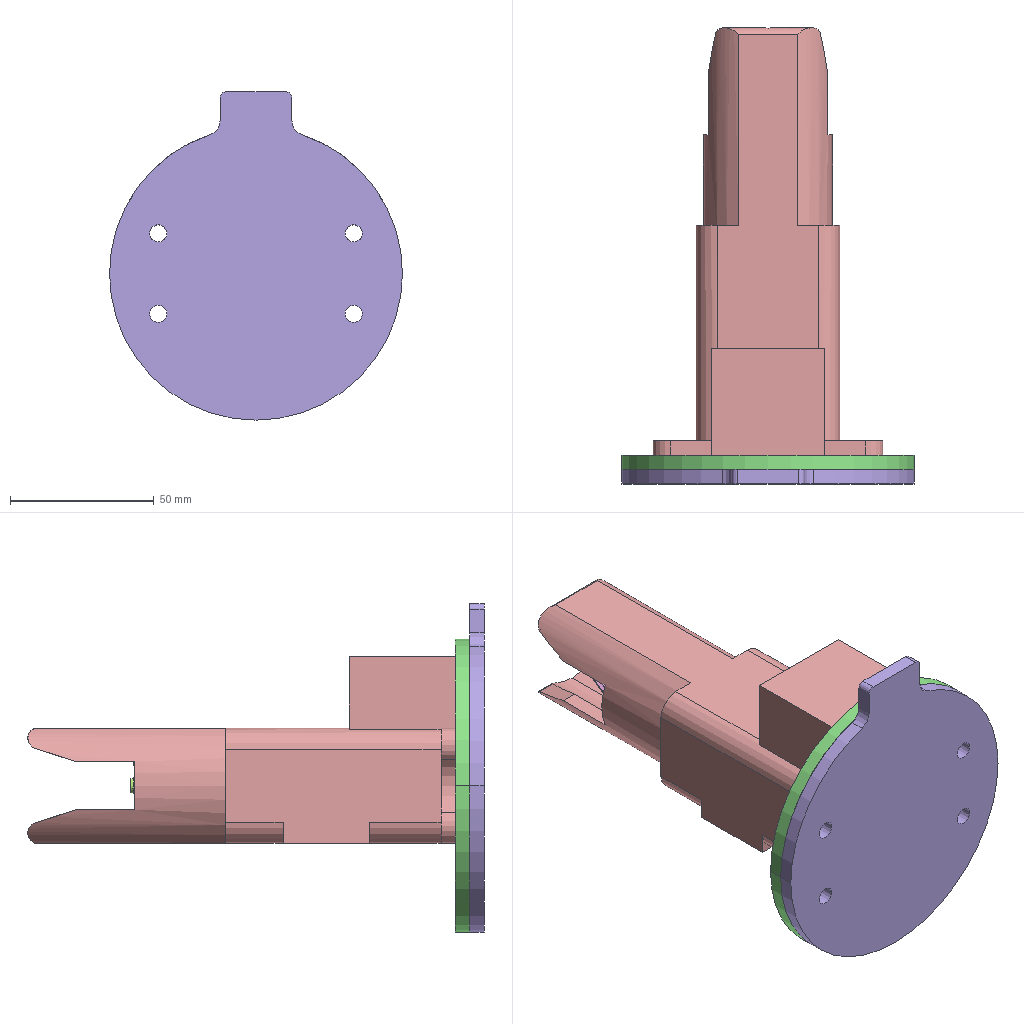Assembly | SolidWorks | 11 different items | 11 placed | box 102 x 159 x 114 mm
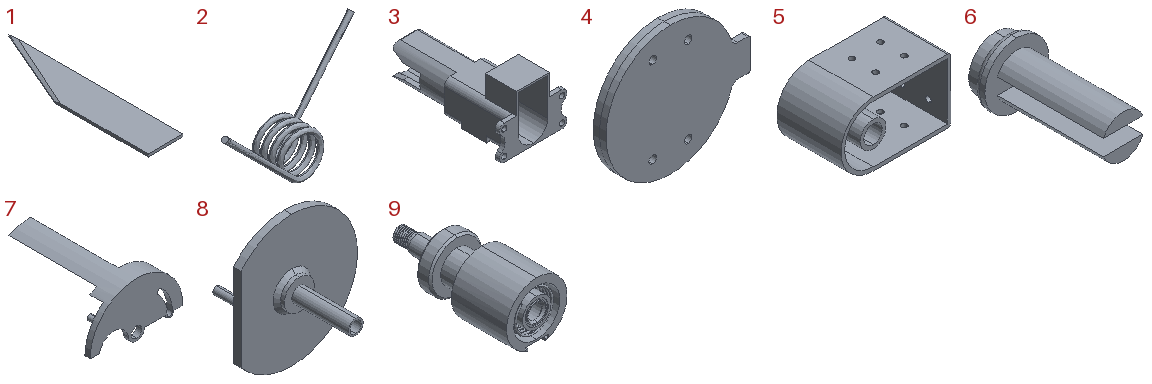Parts list (item | name | quantity | size | volume | features):
1 | - | x1 | 13 x 65 x 1 mm | 641.482 mm3 | features ICE 2, BlendCut 1, Extrusion 1
2 | - | x1 | 21.977 x 6.635 x 10.365 mm | 24.784 mm3 | features MoveFace 2, Helix 1, Sweep 1
3 | - | x1 | 80 x 148.861 x 65 mm | 115092 mm3 | features ICE 22, Extrusion 1, Helix 1, SweepCut 1
4 | - | x1 | 114.307 x 10 x 102 mm | 82051 mm3 | features ICE 4, Extrusion 1, Fillet 1
5 | - | x1 | 60 x 35 x 35 mm | 17116 mm3 | features ICE 5, Extrusion 1, Fillet 1, Shell 1
6 | - | x1 | 6 x 12 x 6 mm | 108.459 mm3 | features ICE 4, Extrusion 1, Fillet 1
7 | - | x1 | 35 x 40 x 20.5 mm | 1485 mm3 | features ICE 20, Chamfer 1, Extrusion 1
8 | - | x1 | 31 x 27 x 35 mm | 2012 mm3 | features ICE 6, Chamfer 1, Extrusion 1
9 | - | x1 | 34 x 77 x 34 mm | 30260 mm3 | features ICE 29, RevCut 6, Chamfer 4, Helix 2, Extrusion 1, Sweep 1, SweepCut 1
10 | angular contact ball bearings gb | x1 | - | - | -
11 | socket head cap screw_ai | x1 | - | - | -
Mates (type | each side: item.copy, entity, surface, feature):
Concentric | 3.1 face cylinder Cut-Extrude1 | 5.1 face cylinder Cut-Extrude1
Coincident | 3.1 face plane Cut-Extrude15 | 5.1 face plane Boss-Extrude1 | 2 times
Coincident | 3.1 face plane Boss-Extrude1 | 4.1 face plane Boss-Extrude3
Concentric | 3.1 face cylinder Cut-Extrude14 | 4.1 face cylinder Cut-Extrude1 | 2 times
Coincident | 9.1 face plane Boss-Extrude7 | 5.1 face plane Boss-Extrude1
Coincident | 9.1 face plane Cut-Extrude29 | 1.1 face plane Boss-Extrude1 | 2 times
Coincident | 9.1 face plane Cut-Extrude28 | 1.1 face plane Boss-Extrude2
Concentric | 9.1 face cylinder Boss-Extrude8 | 5.1 face cylinder Cut-Extrude3
Concentric | 9.1 face cylinder Cut-Revolve7 | 8.1 face cylinder Boss-Extrude3
Coincident | 9.1 face plane Cut-Extrude25 | 8.1 face plane Boss-Extrude1
Concentric | 8.1 face cylinder Boss-Extrude1 | 7.1 face cylinder Boss-Extrude1
Parallel | 1.1 face plane Boss-Extrude1 | 8.1 face plane Cut-Extrude2
Coincident | 8.1 face plane Boss-Extrude1 | 7.1 face plane Cut-Extrude13
Concentric | 6.1 face cylinder Boss-Extrude1 | 8.1 face cylinder Cut-Extrude3
Coincident | 6.1 face plane Boss-Extrude1 | 8.1 face plane Cut-Extrude3
Concentric | 6.1 face cylinder Boss-Extrude1 | 2.1 select_type:24
Coincident | 7.1 face plane Cut-Extrude9 | 2.1 select_type:25
Slot | 7.1 face cylinder Cut-Extrude12 | 8.1 face cylinder Boss-Extrude4